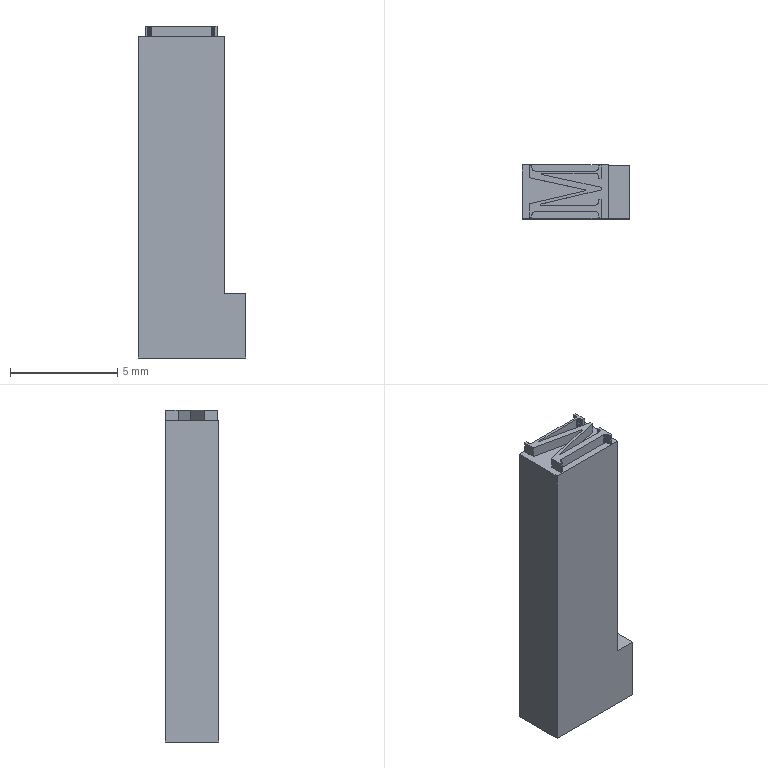Part | NX | features DIE-19 2 | 1 solid | 88 faces | box 5 x 2.5 x 15.5 mm | volume 158.959 mm3 | plane 88